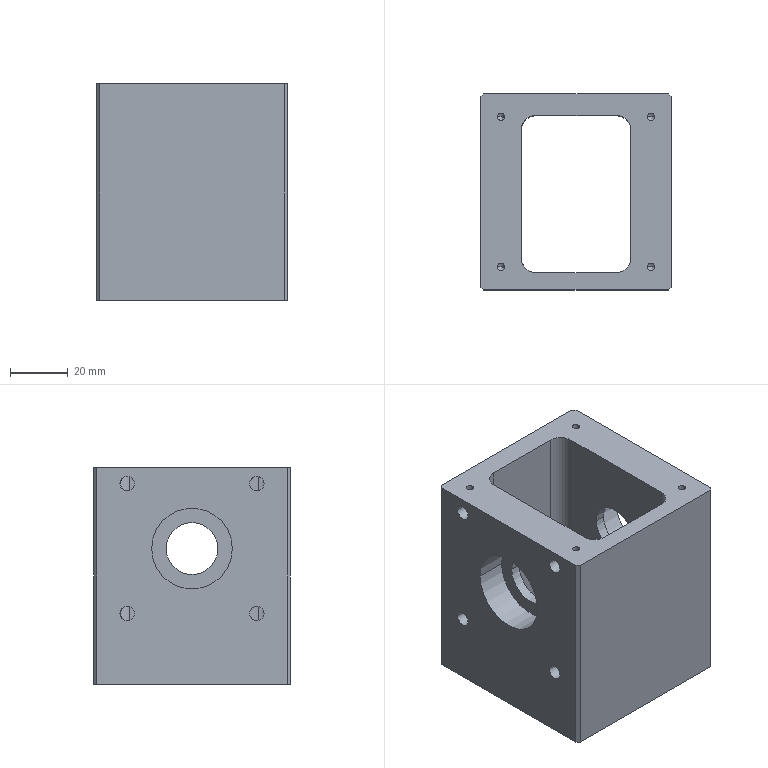Part | SolidWorks | features BaseBody 1 | 1 solid | 78 faces | box 66 x 68 x 75 mm | volume 164943 mm3 | cylinder 40 | cone 22 | plane 16 | commonest cylinder face diameters 5 x16 2.5 x8 6 x4 10 x4 18 x4 28 x4